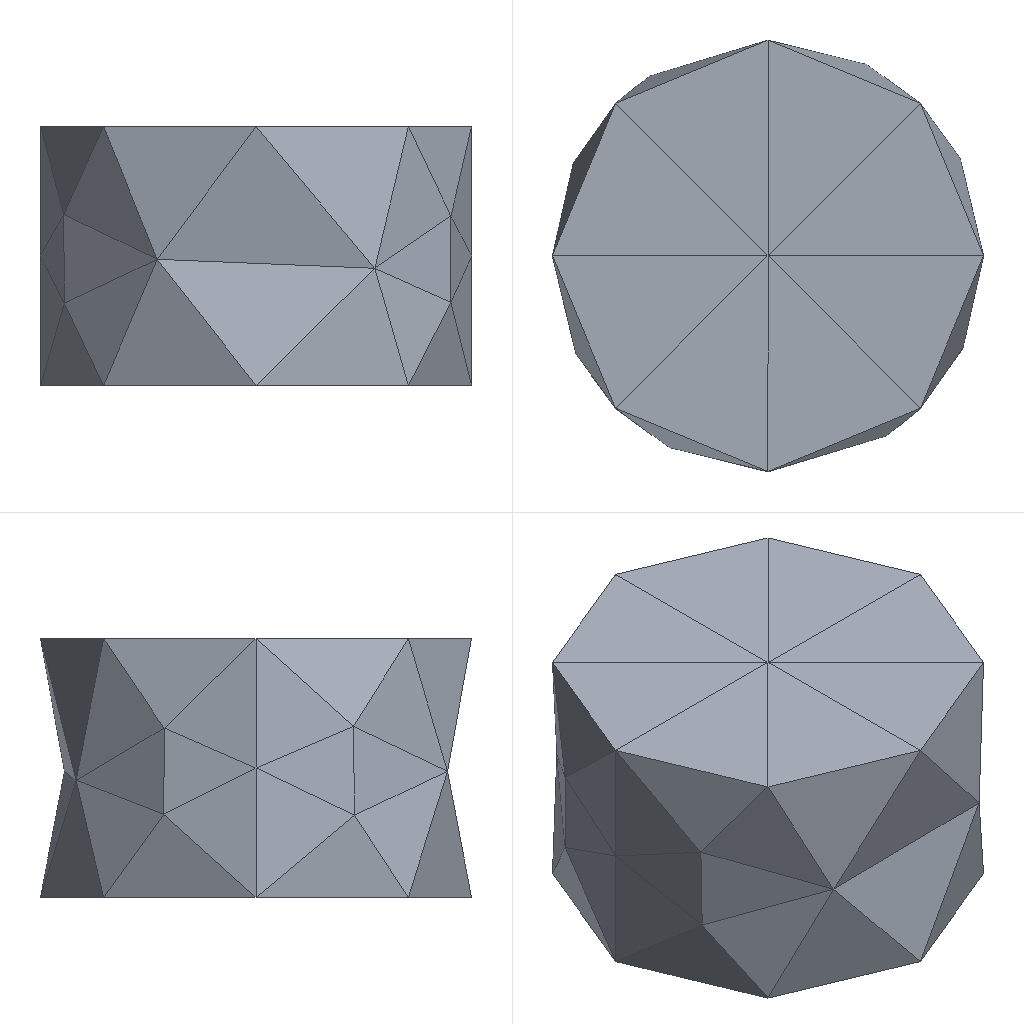Simulation study | ansys mapdl
Set-up summary:
category,name,step,type,value,unit,region
solver,ansys_mapdl
units,mm-N-s-tonne (MPa),,inferred,E=210000 density=
analysis,model,,static
mesh,nodes,,,198
mesh,elements,,,93
element_type,SOLID187,,,93
material,mat 1,,E,210000
material,mat 1,,nu,0.3
load,,model,body load temp,,,all
load,,model,force,"1000 [dir=(0, 0, -1) n=66]",,node list
bc,,model,fixed,"[dofs=UX,UY,UZ n=249]",,node list
Ansys APDL input file, long lists of numbers shortened:
/COM,ANSYS RELEASE 2026 R1           BUILD 26.1      UP20260202       09:09:40
/PREP7
/NOPR
/TITLE,2
ANTYPE, 0
*IF,_CDRDOFF,EQ,1,THEN     !if solid model was read in
_CDRDOFF=             !reset flag, numoffs already performed
*ELSE              !offset database for the following FE model
NUMOFF,NODE,      198
NUMOFF,ELEM,       93
NUMOFF,MAT ,        1
NUMOFF,TYPE,        1
*ENDIF
*SET,_RETURN ,  0.
*SET,_STATUS ,  0.
*SET,_UIQR   ,  66.
*SET,__FLOATPARAMETER__,  198.
DOF,DELETE
ETBLOCK,        1,        1
(2i9,19a9)
        1      187        0        0        0        0        0        0        0        0        0        0        0        0        0        0        0        0        0        0        0
       -1
NBLOCK,6,SOLID,       198,       198
(3i9,6e21.13e3)
        1        0        0-8.8817841970013E-016 1.1000000000000E+000 5.0000000000000E+001
! (197 more lines like these left out)
N,UNBL,LOC,       -1,
EBLOCK,19,SOLID,        93,        93
(19i10)
         1         1         1         1         0         0         0         0        10         0         1       123       121        52         6       129       104       130       131
! (185 more lines like these left out)
        -1
MPTEMP,UNBL, 1, 1,  0.    ,
MPDATA,UNBL, 1,EX  ,       1, 1,  210000.000    ,
MPTEMP,UNBL, 1, 1,  0.    ,
MPDATA,UNBL, 1,NUXY,       1, 1, 0.3    ,
MPTEMP,UNBL, 1, 1,  0.    ,
MPDATA,UNBL, 1,PRXY,       1, 1, 0.3    ,
EXTOPT,ATTR,      0,      0,      0
EXTOPT,ESIZE,  0,  0.
EXTOPT,ACLEAR,      0
TREF,  0.
IRLF,  0
BFUNIF,TEMP,_TINY
ACEL,  0.    ,  0.    ,  0.
OMEGA,  0.    ,  0.    ,  0.
DOMEGA,  0.    ,  0.    ,  0.
CGLOC,  0.    ,  0.    ,  0.
CGOMEGA,  0.    ,  0.    ,  0.
DCGOMG,  0.    ,  0.    ,  0.
KUSE,     0
TIME,  0.
ALPHAD,  0.
BETAD,  0.
DMPRAT,  0.
DMPSTR,  0.
CRPLIM, 0.1    ,   0
CRPLIM,  0.    ,   1
NCNV,     0, 1.000000000E+12,     0,  0.    ,  0.
NEQIT,     0
ERESX,DEFA
DBLOCK,       249
(i9,a6,2(pg16.9))
        1  UX    0.00000000      0.00000000
! (248 more lines like these left out)
       -1
FBLOCK,        66
(i9,a6,2(pg16.9))
       26  FZ   -15.1515152      0.00000000
! (65 more lines like these left out)
       -1
/GO
FINISH
Results summary:
result,analysis_type_db,,,static,unstated
result,n_sets,,,1,unstated
result,load_steps[0].set,load_step=1,,1,unstated
result,load_steps[0].substep,load_step=1,,1,unstated
result,load_steps[0].time,load_step=1,,1,unstated
result,load_steps[0].freq,load_step=1,,1,unstated
result,load_steps[0].max_usum,load_step=1,,0.0002326,unstated
result,load_steps[0].max_seqv,load_step=1,,5.438,unstated
result,load_steps[0].reaction_sum.FX,load_step=1,,6.00409e-13,unstated
result,load_steps[0].reaction_sum.FY,load_step=1,,9.63674e-13,unstated
result,load_steps[0].reaction_sum.FZ,load_step=1,,1000,unstated
result,load_steps[0].reaction_sum.MX,load_step=1,,0,unstated
result,load_steps[0].reaction_sum.MY,load_step=1,,0,unstated
result,load_steps[0].reaction_sum.MZ,load_step=1,,0,unstated
result,convergence,,,results present for all listed sets,unstated